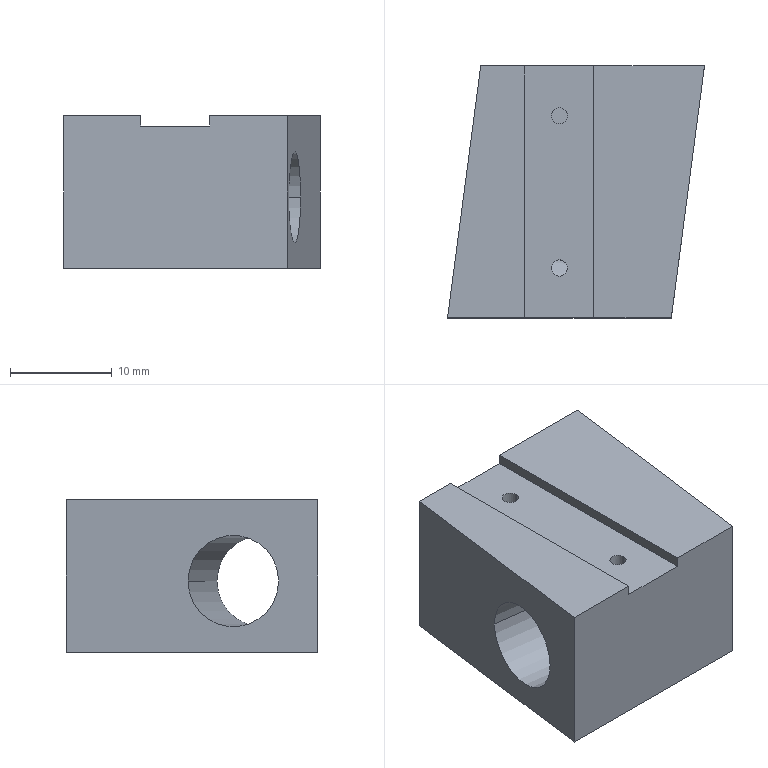Part | SolidWorks | features ICE 4, Extrusion 1 | 1 solid | 17 faces | box 25.3 x 24.8 x 15 mm | volume 6622 mm3 | plane 11 | cylinder 6 | commonest cylinder face diameters 1.6 x4 9 x2
STEP:
#1=CARTESIAN_POINT('',(-9.436,4.918,8.));
#2=VERTEX_POINT('',#1);
#3=CARTESIAN_POINT('',(-7.836,4.918,8.));
#4=VERTEX_POINT('',#3);
#5=CARTESIAN_POINT('',(-8.636,4.918,8.));
#6=DIRECTION('',(0.,0.,1.));
#7=DIRECTION('',(1.,0.,0.));
#8=AXIS2_PLACEMENT_3D('',#5,#6,#7);
#9=CIRCLE('',#8,0.8);
#10=EDGE_CURVE('',#2,#4,#9,.T.);
#11=ORIENTED_EDGE('',*,*,#10,.F.);
#12=CARTESIAN_POINT('',(-9.436,4.918,14.));
#13=VERTEX_POINT('',#12);
#14=CARTESIAN_POINT('',(-9.436,4.918,8.));
#15=DIRECTION('',(0.,0.,1.));
#16=VECTOR('',#15,1000.);
#17=LINE('',#14,#16);
#18=EDGE_CURVE('',#2,#13,#17,.T.);
#19=ORIENTED_EDGE('',*,*,#18,.T.);
#20=CARTESIAN_POINT('',(-7.836,4.918,14.));
#21=VERTEX_POINT('',#20);
#22=CARTESIAN_POINT('',(-8.636,4.918,14.));
#23=DIRECTION('',(0.,0.,1.));
#24=DIRECTION('',(1.,0.,0.));
#25=AXIS2_PLACEMENT_3D('',#22,#23,#24);
#26=CIRCLE('',#25,0.8);
#27=EDGE_CURVE('',#13,#21,#26,.T.);
#28=ORIENTED_EDGE('',*,*,#27,.T.);
#29=CARTESIAN_POINT('',(-7.836,4.918,8.));
#30=DIRECTION('',(0.,0.,1.));
#31=VECTOR('',#30,1000.);
#32=LINE('',#29,#31);
#33=EDGE_CURVE('',#4,#21,#32,.T.);
#34=ORIENTED_EDGE('',*,*,#33,.F.);
#35=EDGE_LOOP('',(#11,#19,#28,#34));
#36=FACE_OUTER_BOUND('',#35,.T.);
#37=CARTESIAN_POINT('',(-8.636,4.918,8.));
#38=DIRECTION('',(0.,0.,1.));
#39=DIRECTION('',(1.,0.,0.));
#40=AXIS2_PLACEMENT_3D('',#37,#38,#39);
#41=CYLINDRICAL_SURFACE('',#40,0.8);
#42=ADVANCED_FACE('',(#36),#41,.F.);
#43=CARTESIAN_POINT('',(-9.436,-10.082,10.919));
#44=VERTEX_POINT('',#43);
#45=CARTESIAN_POINT('',(-7.836,-10.082,11.029));
#46=VERTEX_POINT('',#45);
#47=CARTESIAN_POINT('',(-9.436,-10.082,10.919));
#48=CARTESIAN_POINT('',(-9.436,-10.182,10.863));
#49=CARTESIAN_POINT('',(-9.417,-10.282,10.803));
#50=CARTESIAN_POINT('',(-9.345,-10.466,10.688));
#51=CARTESIAN_POINT('',(-9.291,-10.553,10.63));
#52=CARTESIAN_POINT('',(-9.151,-10.703,10.531));
#53=CARTESIAN_POINT('',(-9.062,-10.769,10.487));
#54=CARTESIAN_POINT('',(-8.856,-10.859,10.435));
#55=CARTESIAN_POINT('',(-8.739,-10.884,10.427));
#56=CARTESIAN_POINT('',(-8.509,-10.88,10.455));
#57=CARTESIAN_POINT('',(-8.399,-10.853,10.49));
#58=CARTESIAN_POINT('',(-8.205,-10.764,10.579));
#59=CARTESIAN_POINT('',(-8.122,-10.703,10.633));
#60=CARTESIAN_POINT('',(-7.915,-10.482,10.805));
#61=CARTESIAN_POINT('',(-7.836,-10.29,10.927));
#62=CARTESIAN_POINT('',(-7.836,-10.082,11.029));
#63=B_SPLINE_CURVE_WITH_KNOTS('',3,(#47,#48,#49,#50,#51,#52,#53,#54,#55,#56,#57,#58,#59,#60,#61,#62),.UNSPECIFIED.,.F.,.F.,(4,2,2,2,2,2,2,4),(0.002614,0.002958,0.003302,0.003645,0.003989,0.004333,0.004677,0.005364),.UNSPECIFIED.);
#64=EDGE_CURVE('',#44,#46,#63,.T.);
#65=ORIENTED_EDGE('',*,*,#64,.F.);
#66=CARTESIAN_POINT('',(-9.436,-10.082,14.));
#67=VERTEX_POINT('',#66);
#68=CARTESIAN_POINT('',(-9.436,-10.082,8.));
#69=DIRECTION('',(0.,0.,1.));
#70=VECTOR('',#69,1000.);
#71=LINE('',#68,#70);
#72=EDGE_CURVE('',#44,#67,#71,.T.);
#73=ORIENTED_EDGE('',*,*,#72,.T.);
#74=CARTESIAN_POINT('',(-7.836,-10.082,14.));
#75=VERTEX_POINT('',#74);
#76=CARTESIAN_POINT('',(-8.636,-10.082,14.));
#77=DIRECTION('',(0.,0.,1.));
#78=DIRECTION('',(1.,0.,0.));
#79=AXIS2_PLACEMENT_3D('',#76,#77,#78);
#80=CIRCLE('',#79,0.8);
#81=EDGE_CURVE('',#67,#75,#80,.T.);
#82=ORIENTED_EDGE('',*,*,#81,.T.);
#83=CARTESIAN_POINT('',(-7.836,-10.082,8.));
#84=DIRECTION('',(0.,0.,1.));
#85=VECTOR('',#84,1000.);
#86=LINE('',#83,#85);
#87=EDGE_CURVE('',#46,#75,#86,.T.);
#88=ORIENTED_EDGE('',*,*,#87,.F.);
#89=EDGE_LOOP('',(#65,#73,#82,#88));
#90=FACE_OUTER_BOUND('',#89,.T.);
#91=CARTESIAN_POINT('',(-8.636,-10.082,8.));
#92=DIRECTION('',(0.,0.,1.));
#93=DIRECTION('',(1.,0.,0.));
#94=AXIS2_PLACEMENT_3D('',#91,#92,#93);
#95=CYLINDRICAL_SURFACE('',#94,0.8);
#96=ADVANCED_FACE('',(#90),#95,.F.);
#97=CARTESIAN_POINT('',(-17.955,-2.192,7.));
#98=VERTEX_POINT('',#97);
#99=CARTESIAN_POINT('',(-19.128,-11.115,7.));
#100=VERTEX_POINT('',#99);
#101=CARTESIAN_POINT('',(-18.541,-6.654,7.));
#102=DIRECTION('',(-0.9915,0.1303,0.));
#103=DIRECTION('',(0.1303,0.9915,0.));
#104=AXIS2_PLACEMENT_3D('',#101,#102,#103);
#105=CIRCLE('',#104,4.5);
#106=EDGE_CURVE('',#98,#100,#105,.T.);
#107=ORIENTED_EDGE('',*,*,#106,.T.);
#108=CARTESIAN_POINT('',(2.538,-13.963,7.));
#109=VERTEX_POINT('',#108);
#110=CARTESIAN_POINT('',(-22.334,-10.694,7.));
#111=DIRECTION('',(0.9915,-0.1303,0.));
#112=VECTOR('',#111,1000.);
#113=LINE('',#110,#112);
#114=EDGE_CURVE('',#100,#109,#113,.T.);
#115=ORIENTED_EDGE('',*,*,#114,.T.);
#116=CARTESIAN_POINT('',(3.711,-5.04,7.));
#117=VERTEX_POINT('',#116);
#118=CARTESIAN_POINT('',(3.124,-9.502,7.));
#119=DIRECTION('',(0.9915,-0.1303,0.));
#120=DIRECTION('',(0.1303,0.9915,0.));
#121=AXIS2_PLACEMENT_3D('',#118,#119,#120);
#122=CIRCLE('',#121,4.5);
#123=EDGE_CURVE('',#109,#117,#122,.T.);
#124=ORIENTED_EDGE('',*,*,#123,.T.);
#125=CARTESIAN_POINT('',(-21.161,-1.771,7.));
#126=DIRECTION('',(0.9915,-0.1303,0.));
#127=VECTOR('',#126,1000.);
#128=LINE('',#125,#127);
#129=EDGE_CURVE('',#98,#117,#128,.T.);
#130=ORIENTED_EDGE('',*,*,#129,.F.);
#131=EDGE_LOOP('',(#107,#115,#124,#130));
#132=FACE_OUTER_BOUND('',#131,.T.);
#133=CARTESIAN_POINT('',(-21.747,-6.232,7.));
#134=DIRECTION('',(0.9915,-0.1303,0.));
#135=DIRECTION('',(0.1303,0.9915,0.));
#136=AXIS2_PLACEMENT_3D('',#133,#134,#135);
#137=CYLINDRICAL_SURFACE('',#136,4.5);
#138=ADVANCED_FACE('',(#132),#137,.F.);
#139=CARTESIAN_POINT('',(-5.236,9.818,15.));
#140=VERTEX_POINT('',#139);
#141=CARTESIAN_POINT('',(-5.236,-14.982,15.));
#142=VERTEX_POINT('',#141);
#143=CARTESIAN_POINT('',(-5.236,9.819,15.));
#144=DIRECTION('',(0.,-1.,0.));
#145=VECTOR('',#144,1000.);
#146=LINE('',#143,#145);
#147=EDGE_CURVE('',#140,#142,#146,.T.);
#148=ORIENTED_EDGE('',*,*,#147,.T.);
#149=CARTESIAN_POINT('',(2.404,-14.982,15.));
#150=VERTEX_POINT('',#149);
#151=CARTESIAN_POINT('',(-19.636,-14.982,15.));
#152=DIRECTION('',(1.,0.,0.));
#153=VECTOR('',#152,1000.);
#154=LINE('',#151,#153);
#155=EDGE_CURVE('',#142,#150,#154,.T.);
#156=ORIENTED_EDGE('',*,*,#155,.T.);
#157=CARTESIAN_POINT('',(5.664,9.818,15.));
#158=VERTEX_POINT('',#157);
#159=CARTESIAN_POINT('',(5.664,9.818,15.));
#160=DIRECTION('',(0.1303,0.9915,0.));
#161=VECTOR('',#160,1000.);
#162=LINE('',#159,#161);
#163=EDGE_CURVE('',#150,#158,#162,.T.);
#164=ORIENTED_EDGE('',*,*,#163,.T.);
#165=CARTESIAN_POINT('',(-19.636,9.818,15.));
#166=DIRECTION('',(-1.,0.,0.));
#167=VECTOR('',#166,1000.);
#168=LINE('',#165,#167);
#169=EDGE_CURVE('',#158,#140,#168,.T.);
#170=ORIENTED_EDGE('',*,*,#169,.T.);
#171=EDGE_LOOP('',(#148,#156,#164,#170));
#172=FACE_OUTER_BOUND('',#171,.T.);
#173=CARTESIAN_POINT('',(0.,0.,15.));
#174=DIRECTION('',(0.,0.,1.));
#175=DIRECTION('',(1.,0.,0.));
#176=AXIS2_PLACEMENT_3D('',#173,#174,#175);
#177=PLANE('',#176);
#178=ADVANCED_FACE('',(#172),#177,.T.);
#179=ORIENTED_EDGE('',*,*,#155,.F.);
#180=CARTESIAN_POINT('',(-5.236,-14.982,14.));
#181=VERTEX_POINT('',#180);
#182=CARTESIAN_POINT('',(-5.236,-14.982,15.));
#183=DIRECTION('',(0.,0.,1.));
#184=VECTOR('',#183,1000.);
#185=LINE('',#182,#184);
#186=EDGE_CURVE('',#181,#142,#185,.T.);
#187=ORIENTED_EDGE('',*,*,#186,.F.);
#188=CARTESIAN_POINT('',(-12.036,-14.982,14.));
#189=VERTEX_POINT('',#188);
#190=CARTESIAN_POINT('',(-5.236,-14.982,14.));
#191=DIRECTION('',(1.,0.,0.));
#192=VECTOR('',#191,1000.);
#193=LINE('',#190,#192);
#194=EDGE_CURVE('',#189,#181,#193,.T.);
#195=ORIENTED_EDGE('',*,*,#194,.F.);
#196=CARTESIAN_POINT('',(-12.036,-14.982,15.));
#197=VERTEX_POINT('',#196);
#198=CARTESIAN_POINT('',(-12.036,-14.982,15.));
#199=DIRECTION('',(0.,0.,-1.));
#200=VECTOR('',#199,1000.);
#201=LINE('',#198,#200);
#202=EDGE_CURVE('',#197,#189,#201,.T.);
#203=ORIENTED_EDGE('',*,*,#202,.F.);
#204=CARTESIAN_POINT('',(-19.636,-14.982,15.));
#205=VERTEX_POINT('',#204);
#206=CARTESIAN_POINT('',(-19.636,-14.982,15.));
#207=DIRECTION('',(1.,0.,0.));
#208=VECTOR('',#207,1000.);
#209=LINE('',#206,#208);
#210=EDGE_CURVE('',#205,#197,#209,.T.);
#211=ORIENTED_EDGE('',*,*,#210,.F.);
#212=CARTESIAN_POINT('',(-19.636,-14.982,0.));
#213=VERTEX_POINT('',#212);
#214=CARTESIAN_POINT('',(-19.636,-14.982,15.));
#215=DIRECTION('',(0.,0.,-1.));
#216=VECTOR('',#215,1000.);
#217=LINE('',#214,#216);
#218=EDGE_CURVE('',#205,#213,#217,.T.);
#219=ORIENTED_EDGE('',*,*,#218,.T.);
#220=CARTESIAN_POINT('',(2.404,-14.982,0.));
#221=VERTEX_POINT('',#220);
#222=CARTESIAN_POINT('',(-19.636,-14.982,0.));
#223=DIRECTION('',(1.,0.,0.));
#224=VECTOR('',#223,1000.);
#225=LINE('',#222,#224);
#226=EDGE_CURVE('',#213,#221,#225,.T.);
#227=ORIENTED_EDGE('',*,*,#226,.T.);
#228=CARTESIAN_POINT('',(2.404,-14.982,15.001));
#229=DIRECTION('',(0.,0.,-1.));
#230=VECTOR('',#229,1000.);
#231=LINE('',#228,#230);
#232=EDGE_CURVE('',#150,#221,#231,.T.);
#233=ORIENTED_EDGE('',*,*,#232,.F.);
#234=EDGE_LOOP('',(#179,#187,#195,#203,#211,#219,#227,#233));
#235=FACE_OUTER_BOUND('',#234,.T.);
#236=CARTESIAN_POINT('',(-19.636,-14.982,15.));
#237=DIRECTION('',(0.,1.,0.));
#238=DIRECTION('',(-1.,0.,0.));
#239=AXIS2_PLACEMENT_3D('',#236,#237,#238);
#240=PLANE('',#239);
#241=ADVANCED_FACE('',(#235),#240,.F.);
#242=CARTESIAN_POINT('',(-5.236,9.818,14.));
#243=VERTEX_POINT('',#242);
#244=CARTESIAN_POINT('',(-12.036,9.818,14.));
#245=VERTEX_POINT('',#244);
#246=CARTESIAN_POINT('',(-5.236,9.818,14.));
#247=DIRECTION('',(-1.,0.,0.));
#248=VECTOR('',#247,1000.);
#249=LINE('',#246,#248);
#250=EDGE_CURVE('',#243,#245,#249,.T.);
#251=ORIENTED_EDGE('',*,*,#250,.F.);
#252=CARTESIAN_POINT('',(-5.236,9.818,15.));
#253=DIRECTION('',(0.,0.,-1.));
#254=VECTOR('',#253,1000.);
#255=LINE('',#252,#254);
#256=EDGE_CURVE('',#140,#243,#255,.T.);
#257=ORIENTED_EDGE('',*,*,#256,.F.);
#258=ORIENTED_EDGE('',*,*,#169,.F.);
#259=CARTESIAN_POINT('',(5.664,9.818,0.));
#260=VERTEX_POINT('',#259);
#261=CARTESIAN_POINT('',(5.664,9.818,15.));
#262=DIRECTION('',(0.,0.,-1.));
#263=VECTOR('',#262,1000.);
#264=LINE('',#261,#263);
#265=EDGE_CURVE('',#158,#260,#264,.T.);
#266=ORIENTED_EDGE('',*,*,#265,.T.);
#267=CARTESIAN_POINT('',(-16.376,9.818,0.));
#268=VERTEX_POINT('',#267);
#269=CARTESIAN_POINT('',(-19.636,9.818,0.));
#270=DIRECTION('',(-1.,0.,0.));
#271=VECTOR('',#270,1000.);
#272=LINE('',#269,#271);
#273=EDGE_CURVE('',#260,#268,#272,.T.);
#274=ORIENTED_EDGE('',*,*,#273,.T.);
#275=CARTESIAN_POINT('',(-16.376,9.818,15.));
#276=VERTEX_POINT('',#275);
#277=CARTESIAN_POINT('',(-16.376,9.818,15.001));
#278=DIRECTION('',(0.,0.,-1.));
#279=VECTOR('',#278,1000.);
#280=LINE('',#277,#279);
#281=EDGE_CURVE('',#276,#268,#280,.T.);
#282=ORIENTED_EDGE('',*,*,#281,.F.);
#283=CARTESIAN_POINT('',(-12.036,9.818,15.));
#284=VERTEX_POINT('',#283);
#285=CARTESIAN_POINT('',(-19.636,9.818,15.));
#286=DIRECTION('',(-1.,0.,0.));
#287=VECTOR('',#286,1000.);
#288=LINE('',#285,#287);
#289=EDGE_CURVE('',#284,#276,#288,.T.);
#290=ORIENTED_EDGE('',*,*,#289,.F.);
#291=CARTESIAN_POINT('',(-12.036,9.818,15.));
#292=DIRECTION('',(0.,0.,1.));
#293=VECTOR('',#292,1000.);
#294=LINE('',#291,#293);
#295=EDGE_CURVE('',#245,#284,#294,.T.);
#296=ORIENTED_EDGE('',*,*,#295,.F.);
#297=EDGE_LOOP('',(#251,#257,#258,#266,#274,#282,#290,#296));
#298=FACE_OUTER_BOUND('',#297,.T.);
#299=CARTESIAN_POINT('',(-19.636,9.818,15.));
#300=DIRECTION('',(0.,-1.,0.));
#301=DIRECTION('',(0.,0.,-1.));
#302=AXIS2_PLACEMENT_3D('',#299,#300,#301);
#303=PLANE('',#302);
#304=ADVANCED_FACE('',(#298),#303,.F.);
#305=CARTESIAN_POINT('',(-12.036,9.819,15.));
#306=DIRECTION('',(0.,-1.,0.));
#307=VECTOR('',#306,1000.);
#308=LINE('',#305,#307);
#309=EDGE_CURVE('',#284,#197,#308,.T.);
#310=ORIENTED_EDGE('',*,*,#309,.F.);
#311=ORIENTED_EDGE('',*,*,#289,.T.);
#312=CARTESIAN_POINT('',(-19.636,-14.982,15.));
#313=DIRECTION('',(-0.1303,-0.9915,0.));
#314=VECTOR('',#313,1000.);
#315=LINE('',#312,#314);
#316=EDGE_CURVE('',#276,#205,#315,.T.);
#317=ORIENTED_EDGE('',*,*,#316,.T.);
#318=ORIENTED_EDGE('',*,*,#210,.T.);
#319=EDGE_LOOP('',(#310,#311,#317,#318));
#320=FACE_OUTER_BOUND('',#319,.T.);
#321=CARTESIAN_POINT('',(0.,0.,15.));
#322=DIRECTION('',(0.,0.,1.));
#323=DIRECTION('',(1.,0.,0.));
#324=AXIS2_PLACEMENT_3D('',#321,#322,#323);
#325=PLANE('',#324);
#326=ADVANCED_FACE('',(#320),#325,.T.);
#327=ORIENTED_EDGE('',*,*,#273,.F.);
#328=CARTESIAN_POINT('',(5.664,9.818,0.));
#329=DIRECTION('',(0.1303,0.9915,0.));
#330=VECTOR('',#329,1000.);
#331=LINE('',#328,#330);
#332=EDGE_CURVE('',#221,#260,#331,.T.);
#333=ORIENTED_EDGE('',*,*,#332,.F.);
#334=ORIENTED_EDGE('',*,*,#226,.F.);
#335=CARTESIAN_POINT('',(-19.636,-14.982,0.));
#336=DIRECTION('',(-0.1303,-0.9915,0.));
#337=VECTOR('',#336,1000.);
#338=LINE('',#335,#337);
#339=EDGE_CURVE('',#268,#213,#338,.T.);
#340=ORIENTED_EDGE('',*,*,#339,.F.);
#341=EDGE_LOOP('',(#327,#333,#334,#340));
#342=FACE_OUTER_BOUND('',#341,.T.);
#343=CARTESIAN_POINT('',(0.,0.,0.));
#344=DIRECTION('',(0.,0.,1.));
#345=DIRECTION('',(1.,0.,0.));
#346=AXIS2_PLACEMENT_3D('',#343,#344,#345);
#347=PLANE('',#346);
#348=ADVANCED_FACE('',(#342),#347,.F.);
#349=ORIENTED_EDGE('',*,*,#106,.F.);
#350=CARTESIAN_POINT('',(-18.541,-6.654,7.));
#351=DIRECTION('',(-0.9915,0.1303,0.));
#352=DIRECTION('',(0.1303,0.9915,0.));
#353=AXIS2_PLACEMENT_3D('',#350,#351,#352);
#354=CIRCLE('',#353,4.5);
#355=EDGE_CURVE('',#100,#98,#354,.T.);
#356=ORIENTED_EDGE('',*,*,#355,.F.);
#357=EDGE_LOOP('',(#349,#356));
#358=FACE_BOUND('',#357,.T.);
#359=ORIENTED_EDGE('',*,*,#281,.T.);
#360=ORIENTED_EDGE('',*,*,#339,.T.);
#361=ORIENTED_EDGE('',*,*,#218,.F.);
#362=ORIENTED_EDGE('',*,*,#316,.F.);
#363=EDGE_LOOP('',(#359,#360,#361,#362));
#364=FACE_OUTER_BOUND('',#363,.T.);
#365=CARTESIAN_POINT('',(-19.636,-14.982,15.001));
#366=DIRECTION('',(0.9915,-0.1303,0.));
#367=DIRECTION('',(0.1303,0.9915,0.));
#368=AXIS2_PLACEMENT_3D('',#365,#366,#367);
#369=PLANE('',#368);
#370=ADVANCED_FACE('',(#358,#364),#369,.F.);
#371=CARTESIAN_POINT('',(3.124,-9.502,7.));
#372=DIRECTION('',(0.9915,-0.1303,0.));
#373=DIRECTION('',(0.1303,0.9915,0.));
#374=AXIS2_PLACEMENT_3D('',#371,#372,#373);
#375=CIRCLE('',#374,4.5);
#376=EDGE_CURVE('',#117,#109,#375,.T.);
#377=ORIENTED_EDGE('',*,*,#376,.F.);
#378=ORIENTED_EDGE('',*,*,#123,.F.);
#379=EDGE_LOOP('',(#377,#378));
#380=FACE_BOUND('',#379,.T.);
#381=ORIENTED_EDGE('',*,*,#232,.T.);
#382=ORIENTED_EDGE('',*,*,#332,.T.);
#383=ORIENTED_EDGE('',*,*,#265,.F.);
#384=ORIENTED_EDGE('',*,*,#163,.F.);
#385=EDGE_LOOP('',(#381,#382,#383,#384));
#386=FACE_OUTER_BOUND('',#385,.T.);
#387=CARTESIAN_POINT('',(5.664,9.818,15.001));
#388=DIRECTION('',(-0.9915,0.1303,0.));
#389=DIRECTION('',(-0.1303,-0.9915,0.));
#390=AXIS2_PLACEMENT_3D('',#387,#388,#389);
#391=PLANE('',#390);
#392=ADVANCED_FACE('',(#380,#386),#391,.F.);
#393=ORIENTED_EDGE('',*,*,#256,.T.);
#394=CARTESIAN_POINT('',(-5.236,9.819,14.));
#395=DIRECTION('',(0.,-1.,0.));
#396=VECTOR('',#395,1000.);
#397=LINE('',#394,#396);
#398=EDGE_CURVE('',#243,#181,#397,.T.);
#399=ORIENTED_EDGE('',*,*,#398,.T.);
#400=ORIENTED_EDGE('',*,*,#186,.T.);
#401=ORIENTED_EDGE('',*,*,#147,.F.);
#402=EDGE_LOOP('',(#393,#399,#400,#401));
#403=FACE_OUTER_BOUND('',#402,.T.);
#404=CARTESIAN_POINT('',(-5.236,9.819,15.));
#405=DIRECTION('',(1.,0.,0.));
#406=DIRECTION('',(0.,1.,0.));
#407=AXIS2_PLACEMENT_3D('',#404,#405,#406);
#408=PLANE('',#407);
#409=ADVANCED_FACE('',(#403),#408,.F.);
#410=CARTESIAN_POINT('',(-8.636,4.918,14.));
#411=DIRECTION('',(0.,0.,1.));
#412=DIRECTION('',(1.,0.,0.));
#413=AXIS2_PLACEMENT_3D('',#410,#411,#412);
#414=CIRCLE('',#413,0.8);
#415=EDGE_CURVE('',#21,#13,#414,.T.);
#416=ORIENTED_EDGE('',*,*,#415,.F.);
#417=ORIENTED_EDGE('',*,*,#27,.F.);
#418=EDGE_LOOP('',(#416,#417));
#419=FACE_BOUND('',#418,.T.);
#420=CARTESIAN_POINT('',(-8.636,-10.082,14.));
#421=DIRECTION('',(0.,0.,1.));
#422=DIRECTION('',(1.,0.,0.));
#423=AXIS2_PLACEMENT_3D('',#420,#421,#422);
#424=CIRCLE('',#423,0.8);
#425=EDGE_CURVE('',#75,#67,#424,.T.);
#426=ORIENTED_EDGE('',*,*,#425,.F.);
#427=ORIENTED_EDGE('',*,*,#81,.F.);
#428=EDGE_LOOP('',(#426,#427));
#429=FACE_BOUND('',#428,.T.);
#430=ORIENTED_EDGE('',*,*,#250,.T.);
#431=CARTESIAN_POINT('',(-12.036,9.819,14.));
#432=DIRECTION('',(0.,-1.,0.));
#433=VECTOR('',#432,1000.);
#434=LINE('',#431,#433);
#435=EDGE_CURVE('',#245,#189,#434,.T.);
#436=ORIENTED_EDGE('',*,*,#435,.T.);
#437=ORIENTED_EDGE('',*,*,#194,.T.);
#438=ORIENTED_EDGE('',*,*,#398,.F.);
#439=EDGE_LOOP('',(#430,#436,#437,#438));
#440=FACE_OUTER_BOUND('',#439,.T.);
#441=CARTESIAN_POINT('',(-5.236,9.819,14.));
#442=DIRECTION('',(0.,0.,-1.));
#443=DIRECTION('',(-1.,0.,0.));
#444=AXIS2_PLACEMENT_3D('',#441,#442,#443);
#445=PLANE('',#444);
#446=ADVANCED_FACE('',(#419,#429,#440),#445,.F.);
#447=ORIENTED_EDGE('',*,*,#295,.T.);
#448=ORIENTED_EDGE('',*,*,#309,.T.);
#449=ORIENTED_EDGE('',*,*,#202,.T.);
#450=ORIENTED_EDGE('',*,*,#435,.F.);
#451=EDGE_LOOP('',(#447,#448,#449,#450));
#452=FACE_OUTER_BOUND('',#451,.T.);
#453=CARTESIAN_POINT('',(-12.036,9.819,15.));
#454=DIRECTION('',(-1.,0.,0.));
#455=DIRECTION('',(0.,-1.,0.));
#456=AXIS2_PLACEMENT_3D('',#453,#454,#455);
#457=PLANE('',#456);
#458=ADVANCED_FACE('',(#452),#457,.F.);
#459=ORIENTED_EDGE('',*,*,#114,.F.);
#460=ORIENTED_EDGE('',*,*,#355,.T.);
#461=ORIENTED_EDGE('',*,*,#129,.T.);
#462=ORIENTED_EDGE('',*,*,#376,.T.);
#463=EDGE_LOOP('',(#459,#460,#461,#462));
#464=FACE_OUTER_BOUND('',#463,.T.);
#465=CARTESIAN_POINT('',(-7.836,-10.082,11.029));
#466=CARTESIAN_POINT('',(-7.836,-9.983,11.078));
#467=CARTESIAN_POINT('',(-7.854,-9.883,11.121));
#468=CARTESIAN_POINT('',(-7.93,-9.691,11.196));
#469=CARTESIAN_POINT('',(-7.988,-9.601,11.226));
#470=CARTESIAN_POINT('',(-8.137,-9.448,11.273));
#471=CARTESIAN_POINT('',(-8.228,-9.385,11.288));
#472=CARTESIAN_POINT('',(-8.429,-9.302,11.306));
#473=CARTESIAN_POINT('',(-8.54,-9.28,11.308));
#474=CARTESIAN_POINT('',(-8.758,-9.284,11.298));
#475=CARTESIAN_POINT('',(-8.866,-9.308,11.286));
#476=CARTESIAN_POINT('',(-9.064,-9.397,11.248));
#477=CARTESIAN_POINT('',(-9.152,-9.461,11.222));
#478=CARTESIAN_POINT('',(-9.365,-9.691,11.121));
#479=CARTESIAN_POINT('',(-9.436,-9.892,11.025));
#480=CARTESIAN_POINT('',(-9.436,-10.082,10.919));
#481=B_SPLINE_CURVE_WITH_KNOTS('',3,(#465,#466,#467,#468,#469,#470,#471,#472,#473,#474,#475,#476,#477,#478,#479,#480),.UNSPECIFIED.,.F.,.F.,(4,2,2,2,2,2,2,4),(0.,0.0003268,0.0006536,0.0009804,0.001307,0.001634,0.001961,0.002614),.UNSPECIFIED.);
#482=EDGE_CURVE('',#46,#44,#481,.T.);
#483=ORIENTED_EDGE('',*,*,#482,.T.);
#484=ORIENTED_EDGE('',*,*,#64,.T.);
#485=EDGE_LOOP('',(#483,#484));
#486=FACE_BOUND('',#485,.T.);
#487=CARTESIAN_POINT('',(-21.747,-6.232,7.));
#488=DIRECTION('',(0.9915,-0.1303,0.));
#489=DIRECTION('',(0.1303,0.9915,0.));
#490=AXIS2_PLACEMENT_3D('',#487,#488,#489);
#491=CYLINDRICAL_SURFACE('',#490,4.5);
#492=ADVANCED_FACE('',(#464,#486),#491,.F.);
#493=ORIENTED_EDGE('',*,*,#72,.F.);
#494=ORIENTED_EDGE('',*,*,#482,.F.);
#495=ORIENTED_EDGE('',*,*,#87,.T.);
#496=ORIENTED_EDGE('',*,*,#425,.T.);
#497=EDGE_LOOP('',(#493,#494,#495,#496));
#498=FACE_OUTER_BOUND('',#497,.T.);
#499=CARTESIAN_POINT('',(-8.636,-10.082,8.));
#500=DIRECTION('',(0.,0.,1.));
#501=DIRECTION('',(1.,0.,0.));
#502=AXIS2_PLACEMENT_3D('',#499,#500,#501);
#503=CYLINDRICAL_SURFACE('',#502,0.8);
#504=ADVANCED_FACE('',(#498),#503,.F.);
#505=ORIENTED_EDGE('',*,*,#18,.F.);
#506=CARTESIAN_POINT('',(-8.636,4.918,8.));
#507=DIRECTION('',(0.,0.,1.));
#508=DIRECTION('',(1.,0.,0.));
#509=AXIS2_PLACEMENT_3D('',#506,#507,#508);
#510=CIRCLE('',#509,0.8);
#511=EDGE_CURVE('',#4,#2,#510,.T.);
#512=ORIENTED_EDGE('',*,*,#511,.F.);
#513=ORIENTED_EDGE('',*,*,#33,.T.);
#514=ORIENTED_EDGE('',*,*,#415,.T.);
#515=EDGE_LOOP('',(#505,#512,#513,#514));
#516=FACE_OUTER_BOUND('',#515,.T.);
#517=CARTESIAN_POINT('',(-8.636,4.918,8.));
#518=DIRECTION('',(0.,0.,1.));
#519=DIRECTION('',(1.,0.,0.));
#520=AXIS2_PLACEMENT_3D('',#517,#518,#519);
#521=CYLINDRICAL_SURFACE('',#520,0.8);
#522=ADVANCED_FACE('',(#516),#521,.F.);
#523=ORIENTED_EDGE('',*,*,#511,.T.);
#524=ORIENTED_EDGE('',*,*,#10,.T.);
#525=EDGE_LOOP('',(#523,#524));
#526=FACE_OUTER_BOUND('',#525,.T.);
#527=CARTESIAN_POINT('',(-8.636,4.918,8.));
#528=DIRECTION('',(0.,0.,1.));
#529=DIRECTION('',(1.,0.,0.));
#530=AXIS2_PLACEMENT_3D('',#527,#528,#529);
#531=PLANE('',#530);
#532=ADVANCED_FACE('',(#526),#531,.T.);
#533=CLOSED_SHELL('',(#42,#96,#138,#178,#241,#304,#326,#348,#370,#392,#409,#446,#458,#492,#504,#522,#532));
#534=MANIFOLD_SOLID_BREP('',#533);
#535=CARTESIAN_POINT('',(0.,0.,0.));
#536=DIRECTION('',(0.,0.,1.));
#537=DIRECTION('',(1.,0.,0.));
#538=AXIS2_PLACEMENT_3D('',#535,#536,#537);
#539=(LENGTH_UNIT()NAMED_UNIT(*)SI_UNIT(.MILLI.,.METRE.));
#540=UNCERTAINTY_MEASURE_WITH_UNIT(LENGTH_MEASURE(0.00001),#539,'','');
#541=(NAMED_UNIT(*)PLANE_ANGLE_UNIT()SI_UNIT($,.RADIAN.));
#542=(NAMED_UNIT(*)SI_UNIT($,.STERADIAN.)SOLID_ANGLE_UNIT());
#543=(GEOMETRIC_REPRESENTATION_CONTEXT(3)GLOBAL_UNCERTAINTY_ASSIGNED_CONTEXT((#540))GLOBAL_UNIT_ASSIGNED_CONTEXT((#539,#541,#542))REPRESENTATION_CONTEXT('',''));
#544=ADVANCED_BREP_SHAPE_REPRESENTATION('',(#534,#538),#543);